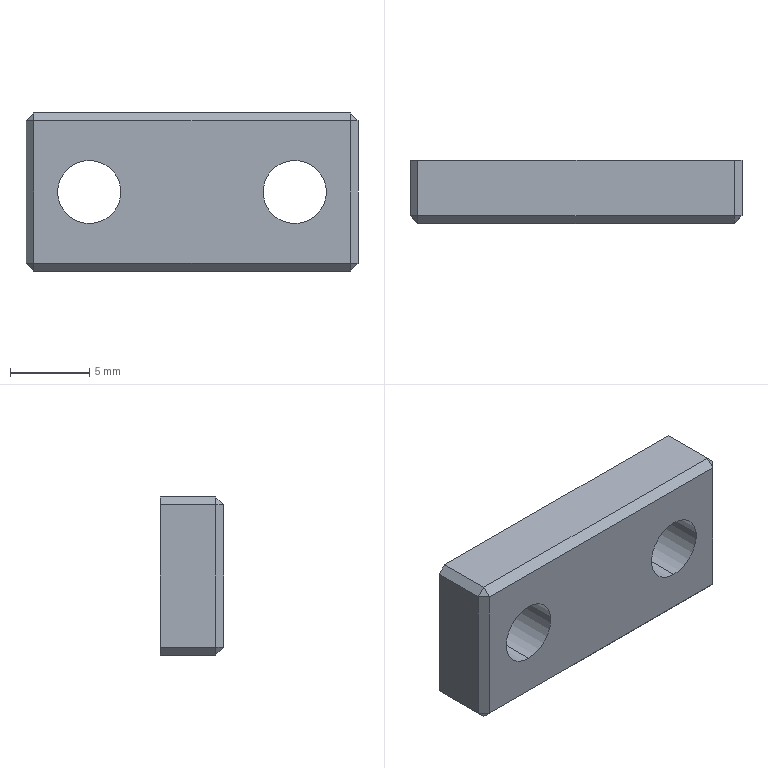Part | SolidWorks | features Chamfer 1, Extrusion 1, ICE 1 | 1 solid | 22 faces | box 21 x 4 x 10 mm | volume 730.052 mm3 | plane 18 | cylinder 4 | commonest cylinder face diameters 4 x4
STEP:
#1=CARTESIAN_POINT('',(17.,-4.,3.));
#2=VERTEX_POINT('',#1);
#3=CARTESIAN_POINT('',(17.,-4.,7.));
#4=VERTEX_POINT('',#3);
#5=CARTESIAN_POINT('',(17.,-4.,5.));
#6=DIRECTION('',(0.,1.,0.));
#7=DIRECTION('',(0.,0.,1.));
#8=AXIS2_PLACEMENT_3D('',#5,#6,#7);
#9=CIRCLE('',#8,2.);
#10=EDGE_CURVE('',#2,#4,#9,.T.);
#11=ORIENTED_EDGE('',*,*,#10,.F.);
#12=CARTESIAN_POINT('',(17.,0.,3.));
#13=VERTEX_POINT('',#12);
#14=CARTESIAN_POINT('',(17.,-10.,3.));
#15=DIRECTION('',(0.,1.,0.));
#16=VECTOR('',#15,1000.);
#17=LINE('',#14,#16);
#18=EDGE_CURVE('',#2,#13,#17,.T.);
#19=ORIENTED_EDGE('',*,*,#18,.T.);
#20=CARTESIAN_POINT('',(17.,0.,7.));
#21=VERTEX_POINT('',#20);
#22=CARTESIAN_POINT('',(17.,0.,5.));
#23=DIRECTION('',(0.,1.,0.));
#24=DIRECTION('',(0.,0.,1.));
#25=AXIS2_PLACEMENT_3D('',#22,#23,#24);
#26=CIRCLE('',#25,2.);
#27=EDGE_CURVE('',#13,#21,#26,.T.);
#28=ORIENTED_EDGE('',*,*,#27,.T.);
#29=CARTESIAN_POINT('',(17.,-10.,7.));
#30=DIRECTION('',(0.,1.,0.));
#31=VECTOR('',#30,1000.);
#32=LINE('',#29,#31);
#33=EDGE_CURVE('',#4,#21,#32,.T.);
#34=ORIENTED_EDGE('',*,*,#33,.F.);
#35=EDGE_LOOP('',(#11,#19,#28,#34));
#36=FACE_OUTER_BOUND('',#35,.T.);
#37=CARTESIAN_POINT('',(17.,-10.,5.));
#38=DIRECTION('',(0.,1.,0.));
#39=DIRECTION('',(0.,0.,1.));
#40=AXIS2_PLACEMENT_3D('',#37,#38,#39);
#41=CYLINDRICAL_SURFACE('',#40,2.);
#42=ADVANCED_FACE('',(#36),#41,.F.);
#43=CARTESIAN_POINT('',(4.,-4.,3.));
#44=VERTEX_POINT('',#43);
#45=CARTESIAN_POINT('',(4.,-4.,7.));
#46=VERTEX_POINT('',#45);
#47=CARTESIAN_POINT('',(4.,-4.,5.));
#48=DIRECTION('',(0.,1.,0.));
#49=DIRECTION('',(0.,0.,1.));
#50=AXIS2_PLACEMENT_3D('',#47,#48,#49);
#51=CIRCLE('',#50,2.);
#52=EDGE_CURVE('',#44,#46,#51,.T.);
#53=ORIENTED_EDGE('',*,*,#52,.F.);
#54=CARTESIAN_POINT('',(4.,0.,3.));
#55=VERTEX_POINT('',#54);
#56=CARTESIAN_POINT('',(4.,-10.,3.));
#57=DIRECTION('',(0.,1.,0.));
#58=VECTOR('',#57,1000.);
#59=LINE('',#56,#58);
#60=EDGE_CURVE('',#44,#55,#59,.T.);
#61=ORIENTED_EDGE('',*,*,#60,.T.);
#62=CARTESIAN_POINT('',(4.,0.,7.));
#63=VERTEX_POINT('',#62);
#64=CARTESIAN_POINT('',(4.,0.,5.));
#65=DIRECTION('',(0.,1.,0.));
#66=DIRECTION('',(0.,0.,1.));
#67=AXIS2_PLACEMENT_3D('',#64,#65,#66);
#68=CIRCLE('',#67,2.);
#69=EDGE_CURVE('',#55,#63,#68,.T.);
#70=ORIENTED_EDGE('',*,*,#69,.T.);
#71=CARTESIAN_POINT('',(4.,-10.,7.));
#72=DIRECTION('',(0.,1.,0.));
#73=VECTOR('',#72,1000.);
#74=LINE('',#71,#73);
#75=EDGE_CURVE('',#46,#63,#74,.T.);
#76=ORIENTED_EDGE('',*,*,#75,.F.);
#77=EDGE_LOOP('',(#53,#61,#70,#76));
#78=FACE_OUTER_BOUND('',#77,.T.);
#79=CARTESIAN_POINT('',(4.,-10.,5.));
#80=DIRECTION('',(0.,1.,0.));
#81=DIRECTION('',(0.,0.,1.));
#82=AXIS2_PLACEMENT_3D('',#79,#80,#81);
#83=CYLINDRICAL_SURFACE('',#82,2.);
#84=ADVANCED_FACE('',(#78),#83,.F.);
#85=CARTESIAN_POINT('',(0.,0.,9.5));
#86=VERTEX_POINT('',#85);
#87=CARTESIAN_POINT('',(0.,0.,0.5));
#88=VERTEX_POINT('',#87);
#89=CARTESIAN_POINT('',(0.,0.,10.));
#90=DIRECTION('',(0.,0.,-1.));
#91=VECTOR('',#90,1000.);
#92=LINE('',#89,#91);
#93=EDGE_CURVE('',#86,#88,#92,.T.);
#94=ORIENTED_EDGE('',*,*,#93,.T.);
#95=CARTESIAN_POINT('',(0.,-3.5,0.5));
#96=VERTEX_POINT('',#95);
#97=CARTESIAN_POINT('',(0.,0.,0.5));
#98=DIRECTION('',(0.,-1.,0.));
#99=VECTOR('',#98,1000.);
#100=LINE('',#97,#99);
#101=EDGE_CURVE('',#88,#96,#100,.T.);
#102=ORIENTED_EDGE('',*,*,#101,.T.);
#103=CARTESIAN_POINT('',(0.,-3.5,9.5));
#104=VERTEX_POINT('',#103);
#105=CARTESIAN_POINT('',(0.,-3.5,10.));
#106=DIRECTION('',(0.,0.,1.));
#107=VECTOR('',#106,1000.);
#108=LINE('',#105,#107);
#109=EDGE_CURVE('',#96,#104,#108,.T.);
#110=ORIENTED_EDGE('',*,*,#109,.T.);
#111=CARTESIAN_POINT('',(0.,0.,9.5));
#112=DIRECTION('',(0.,1.,0.));
#113=VECTOR('',#112,1000.);
#114=LINE('',#111,#113);
#115=EDGE_CURVE('',#104,#86,#114,.T.);
#116=ORIENTED_EDGE('',*,*,#115,.T.);
#117=EDGE_LOOP('',(#94,#102,#110,#116));
#118=FACE_OUTER_BOUND('',#117,.T.);
#119=CARTESIAN_POINT('',(0.,0.,10.));
#120=DIRECTION('',(1.,0.,0.));
#121=DIRECTION('',(0.,0.,-1.));
#122=AXIS2_PLACEMENT_3D('',#119,#120,#121);
#123=PLANE('',#122);
#124=ADVANCED_FACE('',(#118),#123,.F.);
#125=CARTESIAN_POINT('',(20.5,-4.,9.5));
#126=VERTEX_POINT('',#125);
#127=CARTESIAN_POINT('',(0.5,-4.,9.5));
#128=VERTEX_POINT('',#127);
#129=CARTESIAN_POINT('',(0.,-4.,9.5));
#130=DIRECTION('',(-1.,0.,0.));
#131=VECTOR('',#130,1000.);
#132=LINE('',#129,#131);
#133=EDGE_CURVE('',#126,#128,#132,.T.);
#134=ORIENTED_EDGE('',*,*,#133,.T.);
#135=CARTESIAN_POINT('',(0.5,-4.,0.5));
#136=VERTEX_POINT('',#135);
#137=CARTESIAN_POINT('',(0.5,-4.,10.));
#138=DIRECTION('',(0.,0.,-1.));
#139=VECTOR('',#138,1000.);
#140=LINE('',#137,#139);
#141=EDGE_CURVE('',#128,#136,#140,.T.);
#142=ORIENTED_EDGE('',*,*,#141,.T.);
#143=CARTESIAN_POINT('',(20.5,-4.,0.5));
#144=VERTEX_POINT('',#143);
#145=CARTESIAN_POINT('',(0.,-4.,0.5));
#146=DIRECTION('',(1.,0.,0.));
#147=VECTOR('',#146,1000.);
#148=LINE('',#145,#147);
#149=EDGE_CURVE('',#136,#144,#148,.T.);
#150=ORIENTED_EDGE('',*,*,#149,.T.);
#151=CARTESIAN_POINT('',(20.5,-4.,10.));
#152=DIRECTION('',(0.,0.,1.));
#153=VECTOR('',#152,1000.);
#154=LINE('',#151,#153);
#155=EDGE_CURVE('',#144,#126,#154,.T.);
#156=ORIENTED_EDGE('',*,*,#155,.T.);
#157=EDGE_LOOP('',(#134,#142,#150,#156));
#158=FACE_OUTER_BOUND('',#157,.T.);
#159=CARTESIAN_POINT('',(17.,-4.,5.));
#160=DIRECTION('',(0.,1.,0.));
#161=DIRECTION('',(0.,0.,1.));
#162=AXIS2_PLACEMENT_3D('',#159,#160,#161);
#163=CIRCLE('',#162,2.);
#164=EDGE_CURVE('',#4,#2,#163,.T.);
#165=ORIENTED_EDGE('',*,*,#164,.T.);
#166=ORIENTED_EDGE('',*,*,#10,.T.);
#167=EDGE_LOOP('',(#165,#166));
#168=FACE_BOUND('',#167,.T.);
#169=CARTESIAN_POINT('',(4.,-4.,5.));
#170=DIRECTION('',(0.,1.,0.));
#171=DIRECTION('',(0.,0.,1.));
#172=AXIS2_PLACEMENT_3D('',#169,#170,#171);
#173=CIRCLE('',#172,2.);
#174=EDGE_CURVE('',#46,#44,#173,.T.);
#175=ORIENTED_EDGE('',*,*,#174,.T.);
#176=ORIENTED_EDGE('',*,*,#52,.T.);
#177=EDGE_LOOP('',(#175,#176));
#178=FACE_BOUND('',#177,.T.);
#179=CARTESIAN_POINT('',(0.,-4.,10.));
#180=DIRECTION('',(0.,1.,0.));
#181=DIRECTION('',(0.,0.,1.));
#182=AXIS2_PLACEMENT_3D('',#179,#180,#181);
#183=PLANE('',#182);
#184=ADVANCED_FACE('',(#158,#168,#178),#183,.F.);
#185=CARTESIAN_POINT('',(21.,-3.5,9.5));
#186=VERTEX_POINT('',#185);
#187=CARTESIAN_POINT('',(21.,-3.5,0.5));
#188=VERTEX_POINT('',#187);
#189=CARTESIAN_POINT('',(21.,-3.5,10.));
#190=DIRECTION('',(0.,0.,-1.));
#191=VECTOR('',#190,1000.);
#192=LINE('',#189,#191);
#193=EDGE_CURVE('',#186,#188,#192,.T.);
#194=ORIENTED_EDGE('',*,*,#193,.T.);
#195=CARTESIAN_POINT('',(21.,0.,0.5));
#196=VERTEX_POINT('',#195);
#197=CARTESIAN_POINT('',(21.,0.,0.5));
#198=DIRECTION('',(0.,1.,0.));
#199=VECTOR('',#198,1000.);
#200=LINE('',#197,#199);
#201=EDGE_CURVE('',#188,#196,#200,.T.);
#202=ORIENTED_EDGE('',*,*,#201,.T.);
#203=CARTESIAN_POINT('',(21.,0.,9.5));
#204=VERTEX_POINT('',#203);
#205=CARTESIAN_POINT('',(21.,0.,10.));
#206=DIRECTION('',(0.,0.,-1.));
#207=VECTOR('',#206,1000.);
#208=LINE('',#205,#207);
#209=EDGE_CURVE('',#204,#196,#208,.T.);
#210=ORIENTED_EDGE('',*,*,#209,.F.);
#211=CARTESIAN_POINT('',(21.,-4.,9.5));
#212=DIRECTION('',(0.,-1.,0.));
#213=VECTOR('',#212,1000.);
#214=LINE('',#211,#213);
#215=EDGE_CURVE('',#204,#186,#214,.T.);
#216=ORIENTED_EDGE('',*,*,#215,.T.);
#217=EDGE_LOOP('',(#194,#202,#210,#216));
#218=FACE_OUTER_BOUND('',#217,.T.);
#219=CARTESIAN_POINT('',(21.,0.,10.));
#220=DIRECTION('',(-1.,0.,0.));
#221=DIRECTION('',(0.,0.,1.));
#222=AXIS2_PLACEMENT_3D('',#219,#220,#221);
#223=PLANE('',#222);
#224=ADVANCED_FACE('',(#218),#223,.F.);
#225=CARTESIAN_POINT('',(17.,0.,5.));
#226=DIRECTION('',(0.,1.,0.));
#227=DIRECTION('',(0.,0.,1.));
#228=AXIS2_PLACEMENT_3D('',#225,#226,#227);
#229=CIRCLE('',#228,2.);
#230=EDGE_CURVE('',#21,#13,#229,.T.);
#231=ORIENTED_EDGE('',*,*,#230,.F.);
#232=ORIENTED_EDGE('',*,*,#27,.F.);
#233=EDGE_LOOP('',(#231,#232));
#234=FACE_BOUND('',#233,.T.);
#235=CARTESIAN_POINT('',(4.,0.,5.));
#236=DIRECTION('',(0.,1.,0.));
#237=DIRECTION('',(0.,0.,1.));
#238=AXIS2_PLACEMENT_3D('',#235,#236,#237);
#239=CIRCLE('',#238,2.);
#240=EDGE_CURVE('',#63,#55,#239,.T.);
#241=ORIENTED_EDGE('',*,*,#240,.F.);
#242=ORIENTED_EDGE('',*,*,#69,.F.);
#243=EDGE_LOOP('',(#241,#242));
#244=FACE_BOUND('',#243,.T.);
#245=CARTESIAN_POINT('',(20.5,0.,0.));
#246=VERTEX_POINT('',#245);
#247=CARTESIAN_POINT('',(0.5,0.,0.));
#248=VERTEX_POINT('',#247);
#249=CARTESIAN_POINT('',(0.,0.,0.));
#250=DIRECTION('',(-1.,0.,0.));
#251=VECTOR('',#250,1000.);
#252=LINE('',#249,#251);
#253=EDGE_CURVE('',#246,#248,#252,.T.);
#254=ORIENTED_EDGE('',*,*,#253,.T.);
#255=CARTESIAN_POINT('',(0.,0.,0.5));
#256=DIRECTION('',(-0.7071,0.,0.7071));
#257=VECTOR('',#256,1000.);
#258=LINE('',#255,#257);
#259=EDGE_CURVE('',#248,#88,#258,.T.);
#260=ORIENTED_EDGE('',*,*,#259,.T.);
#261=ORIENTED_EDGE('',*,*,#93,.F.);
#262=CARTESIAN_POINT('',(0.5,0.,10.));
#263=VERTEX_POINT('',#262);
#264=CARTESIAN_POINT('',(0.5,0.,10.));
#265=DIRECTION('',(0.7071,0.,0.7071));
#266=VECTOR('',#265,1000.);
#267=LINE('',#264,#266);
#268=EDGE_CURVE('',#86,#263,#267,.T.);
#269=ORIENTED_EDGE('',*,*,#268,.T.);
#270=CARTESIAN_POINT('',(20.5,0.,10.));
#271=VERTEX_POINT('',#270);
#272=CARTESIAN_POINT('',(0.,0.,10.));
#273=DIRECTION('',(-1.,0.,0.));
#274=VECTOR('',#273,1000.);
#275=LINE('',#272,#274);
#276=EDGE_CURVE('',#271,#263,#275,.T.);
#277=ORIENTED_EDGE('',*,*,#276,.F.);
#278=CARTESIAN_POINT('',(20.5,0.,10.));
#279=DIRECTION('',(0.7071,0.,-0.7071));
#280=VECTOR('',#279,1000.);
#281=LINE('',#278,#280);
#282=EDGE_CURVE('',#271,#204,#281,.T.);
#283=ORIENTED_EDGE('',*,*,#282,.T.);
#284=ORIENTED_EDGE('',*,*,#209,.T.);
#285=CARTESIAN_POINT('',(21.,0.,0.5));
#286=DIRECTION('',(-0.7071,0.,-0.7071));
#287=VECTOR('',#286,1000.);
#288=LINE('',#285,#287);
#289=EDGE_CURVE('',#196,#246,#288,.T.);
#290=ORIENTED_EDGE('',*,*,#289,.T.);
#291=EDGE_LOOP('',(#254,#260,#261,#269,#277,#283,#284,#290));
#292=FACE_OUTER_BOUND('',#291,.T.);
#293=CARTESIAN_POINT('',(0.,0.,10.));
#294=DIRECTION('',(0.,-1.,0.));
#295=DIRECTION('',(0.,0.,-1.));
#296=AXIS2_PLACEMENT_3D('',#293,#294,#295);
#297=PLANE('',#296);
#298=ADVANCED_FACE('',(#234,#244,#292),#297,.F.);
#299=CARTESIAN_POINT('',(0.5,-3.5,10.));
#300=VERTEX_POINT('',#299);
#301=CARTESIAN_POINT('',(20.5,-3.5,10.));
#302=VERTEX_POINT('',#301);
#303=CARTESIAN_POINT('',(21.,-3.5,10.));
#304=DIRECTION('',(1.,0.,0.));
#305=VECTOR('',#304,1000.);
#306=LINE('',#303,#305);
#307=EDGE_CURVE('',#300,#302,#306,.T.);
#308=ORIENTED_EDGE('',*,*,#307,.T.);
#309=CARTESIAN_POINT('',(20.5,0.,10.));
#310=DIRECTION('',(0.,1.,0.));
#311=VECTOR('',#310,1000.);
#312=LINE('',#309,#311);
#313=EDGE_CURVE('',#302,#271,#312,.T.);
#314=ORIENTED_EDGE('',*,*,#313,.T.);
#315=ORIENTED_EDGE('',*,*,#276,.T.);
#316=CARTESIAN_POINT('',(0.5,-4.,10.));
#317=DIRECTION('',(0.,-1.,0.));
#318=VECTOR('',#317,1000.);
#319=LINE('',#316,#318);
#320=EDGE_CURVE('',#263,#300,#319,.T.);
#321=ORIENTED_EDGE('',*,*,#320,.T.);
#322=EDGE_LOOP('',(#308,#314,#315,#321));
#323=FACE_OUTER_BOUND('',#322,.T.);
#324=CARTESIAN_POINT('',(0.,0.,10.));
#325=DIRECTION('',(0.,0.,1.));
#326=DIRECTION('',(1.,0.,0.));
#327=AXIS2_PLACEMENT_3D('',#324,#325,#326);
#328=PLANE('',#327);
#329=ADVANCED_FACE('',(#323),#328,.T.);
#330=CARTESIAN_POINT('',(20.5,-3.5,0.));
#331=VERTEX_POINT('',#330);
#332=CARTESIAN_POINT('',(0.5,-3.5,0.));
#333=VERTEX_POINT('',#332);
#334=CARTESIAN_POINT('',(0.,-3.5,0.));
#335=DIRECTION('',(-1.,0.,0.));
#336=VECTOR('',#335,1000.);
#337=LINE('',#334,#336);
#338=EDGE_CURVE('',#331,#333,#337,.T.);
#339=ORIENTED_EDGE('',*,*,#338,.T.);
#340=CARTESIAN_POINT('',(0.5,0.,0.));
#341=DIRECTION('',(0.,1.,0.));
#342=VECTOR('',#341,1000.);
#343=LINE('',#340,#342);
#344=EDGE_CURVE('',#333,#248,#343,.T.);
#345=ORIENTED_EDGE('',*,*,#344,.T.);
#346=ORIENTED_EDGE('',*,*,#253,.F.);
#347=CARTESIAN_POINT('',(20.5,0.,0.));
#348=DIRECTION('',(0.,-1.,0.));
#349=VECTOR('',#348,1000.);
#350=LINE('',#347,#349);
#351=EDGE_CURVE('',#246,#331,#350,.T.);
#352=ORIENTED_EDGE('',*,*,#351,.T.);
#353=EDGE_LOOP('',(#339,#345,#346,#352));
#354=FACE_OUTER_BOUND('',#353,.T.);
#355=CARTESIAN_POINT('',(0.,0.,0.));
#356=DIRECTION('',(0.,0.,1.));
#357=DIRECTION('',(1.,0.,0.));
#358=AXIS2_PLACEMENT_3D('',#355,#356,#357);
#359=PLANE('',#358);
#360=ADVANCED_FACE('',(#354),#359,.F.);
#361=ORIENTED_EDGE('',*,*,#60,.F.);
#362=ORIENTED_EDGE('',*,*,#174,.F.);
#363=ORIENTED_EDGE('',*,*,#75,.T.);
#364=ORIENTED_EDGE('',*,*,#240,.T.);
#365=EDGE_LOOP('',(#361,#362,#363,#364));
#366=FACE_OUTER_BOUND('',#365,.T.);
#367=CARTESIAN_POINT('',(4.,-10.,5.));
#368=DIRECTION('',(0.,1.,0.));
#369=DIRECTION('',(0.,0.,1.));
#370=AXIS2_PLACEMENT_3D('',#367,#368,#369);
#371=CYLINDRICAL_SURFACE('',#370,2.);
#372=ADVANCED_FACE('',(#366),#371,.F.);
#373=ORIENTED_EDGE('',*,*,#18,.F.);
#374=ORIENTED_EDGE('',*,*,#164,.F.);
#375=ORIENTED_EDGE('',*,*,#33,.T.);
#376=ORIENTED_EDGE('',*,*,#230,.T.);
#377=EDGE_LOOP('',(#373,#374,#375,#376));
#378=FACE_OUTER_BOUND('',#377,.T.);
#379=CARTESIAN_POINT('',(17.,-10.,5.));
#380=DIRECTION('',(0.,1.,0.));
#381=DIRECTION('',(0.,0.,1.));
#382=AXIS2_PLACEMENT_3D('',#379,#380,#381);
#383=CYLINDRICAL_SURFACE('',#382,2.);
#384=ADVANCED_FACE('',(#378),#383,.F.);
#385=ORIENTED_EDGE('',*,*,#282,.F.);
#386=ORIENTED_EDGE('',*,*,#313,.F.);
#387=CARTESIAN_POINT('',(20.75,-3.5,9.75));
#388=DIRECTION('',(-0.7071,0.,0.7071));
#389=VECTOR('',#388,1000.);
#390=LINE('',#387,#389);
#391=EDGE_CURVE('',#186,#302,#390,.T.);
#392=ORIENTED_EDGE('',*,*,#391,.F.);
#393=ORIENTED_EDGE('',*,*,#215,.F.);
#394=EDGE_LOOP('',(#385,#386,#392,#393));
#395=FACE_OUTER_BOUND('',#394,.T.);
#396=CARTESIAN_POINT('',(20.5,0.,10.));
#397=DIRECTION('',(0.7071,0.,0.7071));
#398=DIRECTION('',(0.,-1.,0.));
#399=AXIS2_PLACEMENT_3D('',#396,#397,#398);
#400=PLANE('',#399);
#401=ADVANCED_FACE('',(#395),#400,.T.);
#402=CARTESIAN_POINT('',(20.5,-4.,0.5));
#403=DIRECTION('',(-0.7071,-0.7071,0.));
#404=VECTOR('',#403,1000.);
#405=LINE('',#402,#404);
#406=EDGE_CURVE('',#188,#144,#405,.T.);
#407=ORIENTED_EDGE('',*,*,#406,.F.);
#408=ORIENTED_EDGE('',*,*,#193,.F.);
#409=CARTESIAN_POINT('',(20.5,-4.,9.5));
#410=DIRECTION('',(0.7071,0.7071,0.));
#411=VECTOR('',#410,1000.);
#412=LINE('',#409,#411);
#413=EDGE_CURVE('',#126,#186,#412,.T.);
#414=ORIENTED_EDGE('',*,*,#413,.F.);
#415=ORIENTED_EDGE('',*,*,#155,.F.);
#416=EDGE_LOOP('',(#407,#408,#414,#415));
#417=FACE_OUTER_BOUND('',#416,.T.);
#418=CARTESIAN_POINT('',(21.,-3.5,10.));
#419=DIRECTION('',(-0.7071,0.7071,0.));
#420=DIRECTION('',(0.,0.,-1.));
#421=AXIS2_PLACEMENT_3D('',#418,#419,#420);
#422=PLANE('',#421);
#423=ADVANCED_FACE('',(#417),#422,.F.);
#424=ORIENTED_EDGE('',*,*,#289,.F.);
#425=ORIENTED_EDGE('',*,*,#201,.F.);
#426=CARTESIAN_POINT('',(20.75,-3.5,0.25));
#427=DIRECTION('',(0.7071,0.,0.7071));
#428=VECTOR('',#427,1000.);
#429=LINE('',#426,#428);
#430=EDGE_CURVE('',#331,#188,#429,.T.);
#431=ORIENTED_EDGE('',*,*,#430,.F.);
#432=ORIENTED_EDGE('',*,*,#351,.F.);
#433=EDGE_LOOP('',(#424,#425,#431,#432));
#434=FACE_OUTER_BOUND('',#433,.T.);
#435=CARTESIAN_POINT('',(21.,0.,0.5));
#436=DIRECTION('',(-0.7071,0.,0.7071));
#437=DIRECTION('',(0.,1.,0.));
#438=AXIS2_PLACEMENT_3D('',#435,#436,#437);
#439=PLANE('',#438);
#440=ADVANCED_FACE('',(#434),#439,.F.);
#441=ORIENTED_EDGE('',*,*,#413,.T.);
#442=ORIENTED_EDGE('',*,*,#391,.T.);
#443=CARTESIAN_POINT('',(20.5,-4.,9.5));
#444=DIRECTION('',(0.,0.7071,0.7071));
#445=VECTOR('',#444,1000.);
#446=LINE('',#443,#445);
#447=EDGE_CURVE('',#126,#302,#446,.T.);
#448=ORIENTED_EDGE('',*,*,#447,.F.);
#449=EDGE_LOOP('',(#441,#442,#448));
#450=FACE_OUTER_BOUND('',#449,.T.);
#451=CARTESIAN_POINT('',(20.5,-4.,9.5));
#452=DIRECTION('',(0.5774,-0.5774,0.5774));
#453=DIRECTION('',(0.7071,0.,-0.7071));
#454=AXIS2_PLACEMENT_3D('',#451,#452,#453);
#455=PLANE('',#454);
#456=ADVANCED_FACE('',(#450),#455,.T.);
#457=ORIENTED_EDGE('',*,*,#430,.T.);
#458=ORIENTED_EDGE('',*,*,#406,.T.);
#459=CARTESIAN_POINT('',(20.5,-4.,0.5));
#460=DIRECTION('',(0.,-0.7071,0.7071));
#461=VECTOR('',#460,1000.);
#462=LINE('',#459,#461);
#463=EDGE_CURVE('',#331,#144,#462,.T.);
#464=ORIENTED_EDGE('',*,*,#463,.F.);
#465=EDGE_LOOP('',(#457,#458,#464));
#466=FACE_OUTER_BOUND('',#465,.T.);
#467=CARTESIAN_POINT('',(20.5,-4.,0.5));
#468=DIRECTION('',(0.5774,-0.5774,-0.5774));
#469=DIRECTION('',(-0.7071,0.,-0.7071));
#470=AXIS2_PLACEMENT_3D('',#467,#468,#469);
#471=PLANE('',#470);
#472=ADVANCED_FACE('',(#466),#471,.T.);
#473=ORIENTED_EDGE('',*,*,#268,.F.);
#474=ORIENTED_EDGE('',*,*,#115,.F.);
#475=CARTESIAN_POINT('',(0.,-3.5,9.5));
#476=DIRECTION('',(-0.7071,0.,-0.7071));
#477=VECTOR('',#476,1000.);
#478=LINE('',#475,#477);
#479=EDGE_CURVE('',#300,#104,#478,.T.);
#480=ORIENTED_EDGE('',*,*,#479,.F.);
#481=ORIENTED_EDGE('',*,*,#320,.F.);
#482=EDGE_LOOP('',(#473,#474,#480,#481));
#483=FACE_OUTER_BOUND('',#482,.T.);
#484=CARTESIAN_POINT('',(0.5,0.,10.));
#485=DIRECTION('',(-0.7071,0.,0.7071));
#486=DIRECTION('',(0.,1.,0.));
#487=AXIS2_PLACEMENT_3D('',#484,#485,#486);
#488=PLANE('',#487);
#489=ADVANCED_FACE('',(#483),#488,.T.);
#490=ORIENTED_EDGE('',*,*,#447,.T.);
#491=ORIENTED_EDGE('',*,*,#307,.F.);
#492=CARTESIAN_POINT('',(0.5,-3.75,9.75));
#493=DIRECTION('',(0.,0.7071,0.7071));
#494=VECTOR('',#493,1000.);
#495=LINE('',#492,#494);
#496=EDGE_CURVE('',#128,#300,#495,.T.);
#497=ORIENTED_EDGE('',*,*,#496,.F.);
#498=ORIENTED_EDGE('',*,*,#133,.F.);
#499=EDGE_LOOP('',(#490,#491,#497,#498));
#500=FACE_OUTER_BOUND('',#499,.T.);
#501=CARTESIAN_POINT('',(0.,-3.5,10.));
#502=DIRECTION('',(0.,-0.7071,0.7071));
#503=DIRECTION('',(-1.,0.,0.));
#504=AXIS2_PLACEMENT_3D('',#501,#502,#503);
#505=PLANE('',#504);
#506=ADVANCED_FACE('',(#500),#505,.T.);
#507=ORIENTED_EDGE('',*,*,#463,.T.);
#508=ORIENTED_EDGE('',*,*,#149,.F.);
#509=CARTESIAN_POINT('',(0.5,-4.,0.5));
#510=DIRECTION('',(0.,-0.7071,0.7071));
#511=VECTOR('',#510,1000.);
#512=LINE('',#509,#511);
#513=EDGE_CURVE('',#333,#136,#512,.T.);
#514=ORIENTED_EDGE('',*,*,#513,.F.);
#515=ORIENTED_EDGE('',*,*,#338,.F.);
#516=EDGE_LOOP('',(#507,#508,#514,#515));
#517=FACE_OUTER_BOUND('',#516,.T.);
#518=CARTESIAN_POINT('',(0.,-4.,0.5));
#519=DIRECTION('',(0.,0.7071,0.7071));
#520=DIRECTION('',(1.,0.,0.));
#521=AXIS2_PLACEMENT_3D('',#518,#519,#520);
#522=PLANE('',#521);
#523=ADVANCED_FACE('',(#517),#522,.F.);
#524=ORIENTED_EDGE('',*,*,#259,.F.);
#525=ORIENTED_EDGE('',*,*,#344,.F.);
#526=CARTESIAN_POINT('',(0.25,-3.5,0.25));
#527=DIRECTION('',(0.7071,0.,-0.7071));
#528=VECTOR('',#527,1000.);
#529=LINE('',#526,#528);
#530=EDGE_CURVE('',#96,#333,#529,.T.);
#531=ORIENTED_EDGE('',*,*,#530,.F.);
#532=ORIENTED_EDGE('',*,*,#101,.F.);
#533=EDGE_LOOP('',(#524,#525,#531,#532));
#534=FACE_OUTER_BOUND('',#533,.T.);
#535=CARTESIAN_POINT('',(0.,0.,0.5));
#536=DIRECTION('',(0.7071,0.,0.7071));
#537=DIRECTION('',(0.,-1.,0.));
#538=AXIS2_PLACEMENT_3D('',#535,#536,#537);
#539=PLANE('',#538);
#540=ADVANCED_FACE('',(#534),#539,.F.);
#541=ORIENTED_EDGE('',*,*,#496,.T.);
#542=ORIENTED_EDGE('',*,*,#479,.T.);
#543=CARTESIAN_POINT('',(0.,-3.5,9.5));
#544=DIRECTION('',(-0.7071,0.7071,0.));
#545=VECTOR('',#544,1000.);
#546=LINE('',#543,#545);
#547=EDGE_CURVE('',#128,#104,#546,.T.);
#548=ORIENTED_EDGE('',*,*,#547,.F.);
#549=EDGE_LOOP('',(#541,#542,#548));
#550=FACE_OUTER_BOUND('',#549,.T.);
#551=CARTESIAN_POINT('',(0.,-3.5,9.5));
#552=DIRECTION('',(-0.5774,-0.5774,0.5774));
#553=DIRECTION('',(0.7071,0.,0.7071));
#554=AXIS2_PLACEMENT_3D('',#551,#552,#553);
#555=PLANE('',#554);
#556=ADVANCED_FACE('',(#550),#555,.T.);
#557=ORIENTED_EDGE('',*,*,#530,.T.);
#558=ORIENTED_EDGE('',*,*,#513,.T.);
#559=CARTESIAN_POINT('',(0.5,-4.,0.5));
#560=DIRECTION('',(0.7071,-0.7071,0.));
#561=VECTOR('',#560,1000.);
#562=LINE('',#559,#561);
#563=EDGE_CURVE('',#96,#136,#562,.T.);
#564=ORIENTED_EDGE('',*,*,#563,.F.);
#565=EDGE_LOOP('',(#557,#558,#564));
#566=FACE_OUTER_BOUND('',#565,.T.);
#567=CARTESIAN_POINT('',(0.5,-4.,0.5));
#568=DIRECTION('',(-0.5774,-0.5774,-0.5774));
#569=DIRECTION('',(-0.7071,0.,0.7071));
#570=AXIS2_PLACEMENT_3D('',#567,#568,#569);
#571=PLANE('',#570);
#572=ADVANCED_FACE('',(#566),#571,.T.);
#573=ORIENTED_EDGE('',*,*,#547,.T.);
#574=ORIENTED_EDGE('',*,*,#109,.F.);
#575=ORIENTED_EDGE('',*,*,#563,.T.);
#576=ORIENTED_EDGE('',*,*,#141,.F.);
#577=EDGE_LOOP('',(#573,#574,#575,#576));
#578=FACE_OUTER_BOUND('',#577,.T.);
#579=CARTESIAN_POINT('',(0.5,-4.,10.));
#580=DIRECTION('',(0.7071,0.7071,0.));
#581=DIRECTION('',(0.,0.,-1.));
#582=AXIS2_PLACEMENT_3D('',#579,#580,#581);
#583=PLANE('',#582);
#584=ADVANCED_FACE('',(#578),#583,.F.);
#585=CLOSED_SHELL('',(#42,#84,#124,#184,#224,#298,#329,#360,#372,#384,#401,#423,#440,#456,#472,#489,#506,#523,#540,#556,#572,#584));
#586=MANIFOLD_SOLID_BREP('',#585);
#587=CARTESIAN_POINT('',(0.,0.,0.));
#588=DIRECTION('',(0.,0.,1.));
#589=DIRECTION('',(1.,0.,0.));
#590=AXIS2_PLACEMENT_3D('',#587,#588,#589);
#591=(LENGTH_UNIT()NAMED_UNIT(*)SI_UNIT(.MILLI.,.METRE.));
#592=UNCERTAINTY_MEASURE_WITH_UNIT(LENGTH_MEASURE(0.00001),#591,'','');
#593=(NAMED_UNIT(*)PLANE_ANGLE_UNIT()SI_UNIT($,.RADIAN.));
#594=(NAMED_UNIT(*)SI_UNIT($,.STERADIAN.)SOLID_ANGLE_UNIT());
#595=(GEOMETRIC_REPRESENTATION_CONTEXT(3)GLOBAL_UNCERTAINTY_ASSIGNED_CONTEXT((#592))GLOBAL_UNIT_ASSIGNED_CONTEXT((#591,#593,#594))REPRESENTATION_CONTEXT('',''));
#596=ADVANCED_BREP_SHAPE_REPRESENTATION('',(#586,#590),#595);